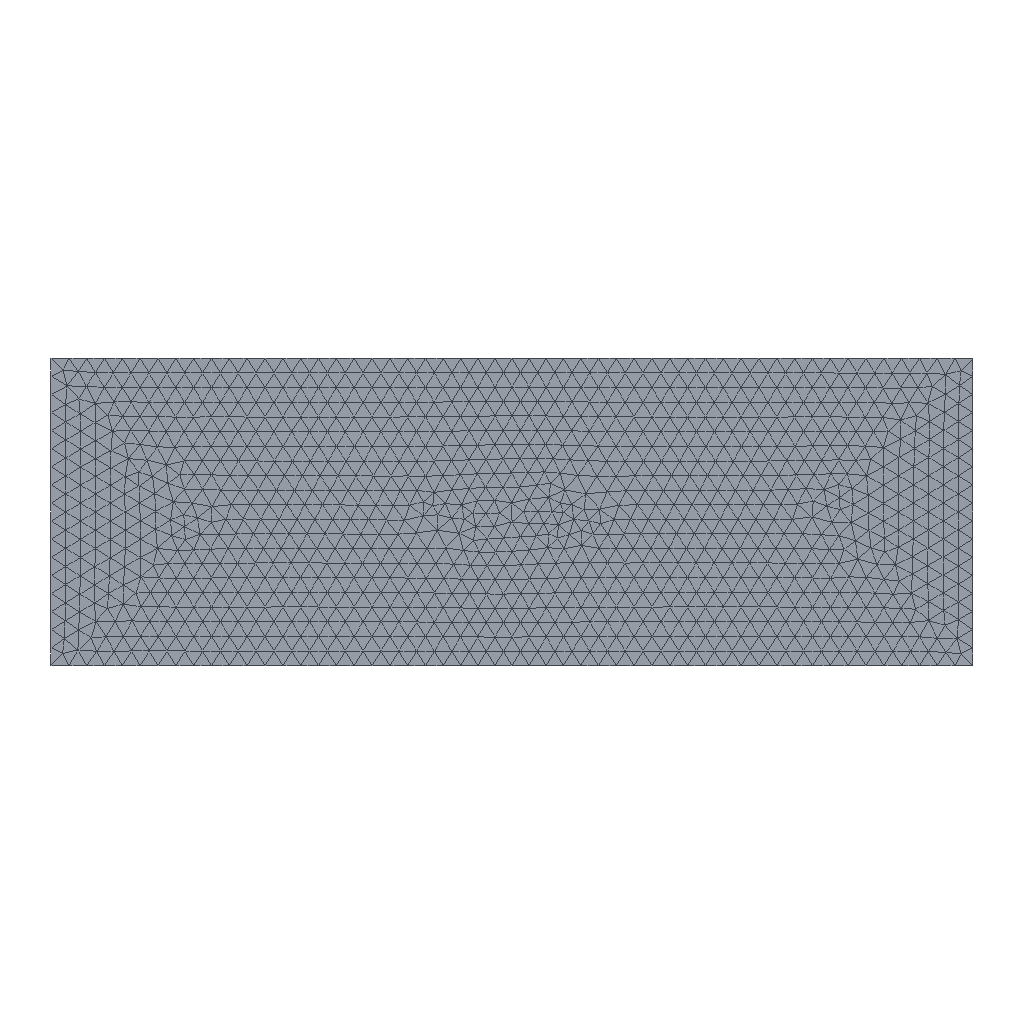Simulation study | comsol
Notes in the study folder:
sigma0 1.04e3[S/m] Silicon conductivity
Rh 1.25e-4[m^3/C] Hall coefficient
Bz 0.1[T] Magnetic field
coeff0 sigma0/(1+(sigma0*Rh*Bz)^2) Conductivity anisotropy 2
V0 5.0[V] Applied voltage
t_Si 1.0e-3[m] Silicon thickness
coeff1 sigma0*Rh*Bz Conductivity anisotropy 1
s11 coeff0 Conductivity matrix term 11
s12 coeff0*coeff1 Conductivity matrix term 12
s21 -coeff0*coeff1 Conductivity matrix term 21
s22 coeff0 Conductivity matrix term 22
epsilon_Si 11.68 Relative permittivity silicon
Set-up summary:
category,name,step,type,value,unit,region
solver,comsol,,COMSOL Multiphysics 6.4 (Build: 293)
units,SI; geometry length unit m,,stated,COMSOL default unit system (SI)
analysis,Study 1,,Parametric + Stationary,space_dimension=2D
load_step,std1/param,std1/param,Parametric + Stationary,"type=Parametric; parameter=Bz; parameter values=range(0,0.1,2); parameter unit=T"
load_step,std1/stat,std1/stat,Parametric + Stationary,type=Stationary
mesh,nodes,,,1181
mesh,elements,,,2222
element_type,tri,,,2222
element_type,edg,,,138
element_type,vtx,,,8
component,mod1,,2D,geometry=geom1; domains=1
physics,Electric Currents (ec),mod1,ConductiveMedia,V(V)
parameter,sigma0,,,1.04e3[S/m]
parameter,Rh,,,1.25e-4[m^3/C]
parameter,Bz,,,0.1[T]
parameter,coeff0,,,sigma0/(1+(sigma0*Rh*Bz)^2)
parameter,V0,,,5.0[V]
parameter,t_Si,,,1.0e-3[m]
parameter,coeff1,,,sigma0*Rh*Bz
parameter,s11,,,coeff0
parameter,s12,,,coeff0*coeff1
parameter,s21,,,-coeff0*coeff1
parameter,s22,,,coeff0
parameter,epsilon_Si,,,11.68
bc,Current Conservation 1 (cucn1),mod1/ec,CurrentConservationSolid,sigma=s11 s21 0 s12 s22 0 0 0 0; rho0=0; Tref=293.15[K]; alpha=0; epsilonr=epsilon_Si; epsilonBis=0; epsilonPrim=1; delta=0; P=0 0 0; Dr=0 0 0; ConstitutiveRelationDE=RelativePermittivity; materialType=solid; ConstitutiveRelationJcE=ElectricalConductivity; HallCoef=0; sigma0=0; HallEffectMagneticFluxDensity=0 0 0; tanDelta=0; epsilonrS=1,,selection [1]
bc,Electric Insulation 1 (ein1),mod1/ec,ElectricInsulation,,,selection []
bc,Initial Values 1 (init1),mod1/ec,init,V=0,,selection [1]
bc,Continuity (dcont1),mod1/ec,Continuity,pairDisconnect=1; nitscheFormulation=skew; applyOn=dst; stabilizationTerm=automatic; stabilizationFactor=1; pairSelection=all; pairsList=0,,selection []
bc,Electric Insulation 2 (ein2),mod1/ec,ElectricInsulation,,,"selection [2, 3, 6, 7]"
bc,Ground 1 (gnd1),mod1/ec,Ground,V0=0,,selection [1]
bc,Electric Potential 1 (pot1),mod1/ec,ElectricPotential,V0=V0,,selection [8]
bc,Floating Potential 1 (fp1),mod1/ec,FloatingPotential,I0=0; Tag=fp1; Group=0; TerminalType=userDefined; Vinit=0[V]; I_cir=0,,selection [5]
bc,Floating Potential 2 (fp2),mod1/ec,FloatingPotential,I0=0; Tag=fp2; Group=0; TerminalType=userDefined; Vinit=0[V]; I_cir=0,,selection [4]
COMSOL model file for Java, long lists of numbers shortened:
/*
 * em_deck.java
 */

import com.comsol.model.*;
import com.comsol.model.util.*;

/** Model exported on Oct 28 2026, 10:33 by COMSOL 6.4.0.293. */
public class em_deck {

  public static Model run() {
    Model model = ModelUtil.create("Model");

    model.modelPath("");

    model.label("in.mph");

    model.param().set("sigma0", "1.04e3[S/m]", "Silicon conductivity");
    model.param().set("Rh", "1.25e-4[m^3/C]", "Hall coefficient");
    model.param().set("Bz", "0.1[T]", "Magnetic field");
    model.param().set("coeff0", "sigma0/(1+(sigma0*Rh*Bz)^2)", "Conductivity anisotropy 2");
    model.param().set("V0", "5.0[V]", "Applied voltage");
    model.param().set("t_Si", "1.0e-3[m]", "Silicon thickness");
    model.param().set("coeff1", "sigma0*Rh*Bz", "Conductivity anisotropy 1");
    model.param().set("s11", "coeff0", "Conductivity matrix term 11");
    model.param().set("s12", "coeff0*coeff1", "Conductivity matrix term 12");
    model.param().set("s21", "-coeff0*coeff1", "Conductivity matrix term 21");
    model.param().set("s22", "coeff0", "Conductivity matrix term 22");
    model.param().set("epsilon_Si", "11.68", "Relative permittivity silicon");

    model.component().create("mod1", false);

    model.component("mod1").geom().create("geom1", 2);

    model.component("mod1").label("Model 1");

    model.component("mod1").defineLocalCoord(false);

    model.component("mod1").curvedInterior(false);

    model.component("mod1").mesh().create("mesh1");

    model.component("mod1").geom("geom1").repairTolType("relative");
    model.component("mod1").geom("geom1").create("r1", "Rectangle");
    model.component("mod1").geom("geom1").feature("r1").set("size", new String[]{"1.8e-2", "6e-3"});
    model.component("mod1").geom("geom1").feature("r1").set("pos", new String[]{"-9e-3", "-3e-3"});
    model.component("mod1").geom("geom1").create("pt1", "Point");
    model.component("mod1").geom("geom1").feature("pt1").set("p", new String[]{"-1e-3", "3e-3"});
    model.component("mod1").geom("geom1").create("pt2", "Point");
    model.component("mod1").geom("geom1").feature("pt2").set("p", new String[]{"1e-3", "3e-3"});
    model.component("mod1").geom("geom1").create("pt3", "Point");
    model.component("mod1").geom("geom1").feature("pt3").set("p", new String[]{"-1e-3", "-3e-3"});
    model.component("mod1").geom("geom1").create("pt4", "Point");
    model.component("mod1").geom("geom1").feature("pt4").set("p", new String[]{"1e-3", "-3e-3"});
    model.component("mod1").geom("geom1").feature("fin").set("repairtoltype", "relative");
    model.component("mod1").geom("geom1").run();

    model.component("mod1").physics().create("ec", "ConductiveMedia", "geom1");
    model.component("mod1").physics("ec").create("cucn1", "CurrentConservationSolid", 2);
    model.component("mod1").physics("ec").feature("cucn1").selection().all();
    model.component("mod1").physics("ec").feature("cucn1").featureInfo().create("information");
    model.component("mod1").physics("ec").create("ein2", "ElectricInsulation", 1);
    model.component("mod1").physics("ec").feature("ein2").selection().set(2, 3, 6, 7);
    model.component("mod1").physics("ec").create("gnd1", "Ground", 1);
    model.component("mod1").physics("ec").feature("gnd1").selection().set(1);
    model.component("mod1").physics("ec").create("pot1", "ElectricPotential", 1);
    model.component("mod1").physics("ec").feature("pot1").selection().set(8);
    model.component("mod1").physics("ec").create("fp1", "FloatingPotential", 1);
    model.component("mod1").physics("ec").feature("fp1").selection().set(5);
    model.component("mod1").physics("ec").create("fp2", "FloatingPotential", 1);
    model.component("mod1").physics("ec").feature("fp2").selection().set(4);

    model.component("mod1").mesh("mesh1").autoMeshSize(2);

    model.thermodynamics().label("Thermodynamics Package");

    model.component("mod1").view("view1").set("showlabels", true);
    model.component("mod1").view("view1").axis().set("xmin", -0.01041);
    model.component("mod1").view("view1").axis().set("xmax", 0.01041);
    model.component("mod1").view("view1").axis().set("ymin", -0.0135);
    model.component("mod1").view("view1").axis().set("ymax", 0.0135);

    model.component("mod1").physics("ec").prop("ShapeProperty").set("frame", "material");
    model.component("mod1").physics("ec").prop("d").set("d", "t_Si");
    model.component("mod1").physics("ec").prop("PortSweepSettings").set("PortParamName", "PortName");
    model.component("mod1").physics("ec").prop("PortSweepSettings").set("zref", 50);
    model.component("mod1").physics("ec").feature("cucn1").set("sigma_mat", "userdef");
    model.component("mod1").physics("ec").feature("cucn1")
         .set("sigma", new String[][]{{"s11"}, {"s21"}, {"0"}, {"s12"}, {"s22"}, {"0"}, {"0"}, {"0"}, {"0"}});
    model.component("mod1").physics("ec").feature("cucn1").set("rho0", 0);
    model.component("mod1").physics("ec").feature("cucn1").set("Tref", "293.15[K]");
    model.component("mod1").physics("ec").feature("cucn1").set("epsilonr_mat", "userdef");
    model.component("mod1").physics("ec").feature("cucn1")
         .set("epsilonr", new String[][]{{"epsilon_Si"}, {"0"}, {"0"}, {"0"}, {"epsilon_Si"}, {"0"}, {"0"}, {"0"}, {"epsilon_Si"}});
    model.component("mod1").physics("ec").feature("cucn1")
         .set("epsilonBis", new int[][]{{0}, {0}, {0}, {0}, {0}, {0}, {0}, {0}, {0}});
    model.component("mod1").physics("ec").feature("cucn1").set("minput_temperature_src", "userdef");
    model.component("mod1").physics("ec").feature("cucn1").set("minput_electricfield_src", "root.mod1.ec.Ex");
    model.component("mod1").physics("ec").feature("cucn1").label("Current Conservation 1");
    model.component("mod1").physics("ec").feature("cucn1").featureInfo("information").label("Migrated Feature");
    model.component("mod1").physics("ec").feature("dcont1").set("pairDisconnect", true);
    model.component("mod1").physics("ec").feature("dcont1").label("Continuity");
    model.component("mod1").physics("ec").feature("gnd1").set("constraintOptions", "weakConstraints");
    model.component("mod1").physics("ec").feature("pot1").set("V0", "V0");
    model.component("mod1").physics("ec").feature("pot1").set("constraintOptions", "weakConstraints");

    model.study().create("std1");
    model.study("std1").create("param", "Parametric");
    model.study("std1").create("stat", "Stationary");

    model.sol().create("sol1");
    model.sol("sol1").attach("std1");
    model.sol("sol1").create("st1", "StudyStep");
    model.sol("sol1").create("v1", "Variables");
    model.sol("sol1").create("s1", "Stationary");
    model.sol("sol1").feature("s1").create("p1", "Parametric");
    model.sol("sol1").feature("s1").create("fc1", "FullyCoupled");
    model.sol("sol1").feature("s1").feature().remove("fcDef");

    model.result().create("pg1", "PlotGroup2D");
    model.result("pg1").create("surf1", "Surface");
    model.result("pg1").create("con1", "Contour");

    model.study("std1").feature("param").set("pname", new String[]{"Bz"});
    model.study("std1").feature("param").set("plistarr", new String[]{"range(0,0.1,2)"});
    model.study("std1").feature("param").set("punit", new String[]{"T"});

    model.sol("sol1").label("Solver 1");
    model.sol("sol1").feature("st1").label("Compile Equations: Stationary");
    model.sol("sol1").feature("v1").label("Dependent Variables 1.1");
    model.sol("sol1").feature("v1").set("clistctrl", new String[]{"p1"});
    model.sol("sol1").feature("v1").set("cname", new String[]{"Bz"});
    model.sol("sol1").feature("v1").set("clist", new String[]{"range(0,0.1,2)"});
    model.sol("sol1").feature("s1").label("Stationary Solver 1.1");
    model.sol("sol1").feature("s1").set("control", "user");
    model.sol("sol1").feature("s1").set("stol", "0.001");
    model.sol("sol1").feature("s1").feature("dDef").label("Direct 1");
    model.sol("sol1").feature("s1").feature("dDef").set("thresh", 0.1);
    model.sol("sol1").feature("s1").feature("dDef").set("ooc", false);
    model.sol("sol1").feature("s1").feature("dDef").set("rhob", 400);
    model.sol("sol1").feature("s1").feature("aDef").label("Advanced 1");
    model.sol("sol1").feature("s1").feature("p1").label("Parametric 1.1");
    model.sol("sol1").feature("s1").feature("p1").set("control", "param");
    model.sol("sol1").feature("s1").feature("p1").set("pname", new String[]{"Bz"});
    model.sol("sol1").feature("s1").feature("p1").set("plistarr", new String[]{"range(0,0.1,2)"});
    model.sol("sol1").feature("s1").feature("p1").set("punit", new String[]{"T"});
    model.sol("sol1").feature("s1").feature("p1").set("continuationlsqall", false);
    model.sol("sol1").feature("s1").feature("fc1").label("Fully Coupled 1.1");
    model.sol("sol1").feature("s1").feature("fc1").set("termonres", false);
    model.sol("sol1").feature("s1").feature("fc1").set("probesel", "manual");

    model.study("std1").runNoGen();

    model.result().dataset("dset1").label("Solution 1");
    model.result().dataset("dset1").set("frametype", "material");
    model.result("pg1").set("smooth", "internal");
    model.result("pg1").feature("surf1").set("colortable", "RainbowClassic");
    model.result("pg1").feature("surf1").set("smooth", "internal");
    model.result("pg1").feature("surf1").set("resolution", "normal");
    model.result("pg1").feature("con1").set("levelrounding", false);
    model.result("pg1").feature("con1").set("colortable", "GrayScale");
    model.result("pg1").feature("con1").set("legendtype", "lines");
    model.result("pg1").feature("con1").set("smooth", "internal");
    model.result("pg1").feature("con1").set("resolution", "normal");

    return model;
  }

  public static void main(String[] args) {
    run();
  }

}
Results summary:
result,max V = abs(mod1.V),dset1 (21 solution(s)),,5,V